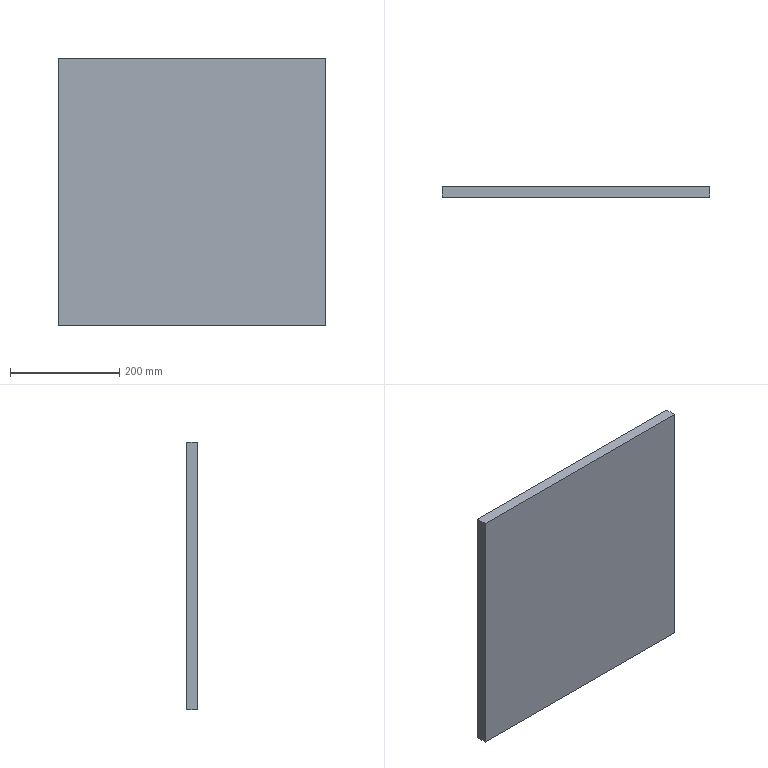Part | STEP file | 1 solid | 6 faces | box 490 x 20 x 490 mm | volume 4802000 mm3 | plane 6
STEP:
#1=CARTESIAN_POINT('',(0.,0.,0.));
#2=DIRECTION('',(0.,0.,1.));
#3=DIRECTION('',(1.,0.,0.));
#4=AXIS2_PLACEMENT_3D('',#1,#2,#3);
#5=CARTESIAN_POINT('',(245.,0.,245.));
#6=VERTEX_POINT('',#5);
#7=CARTESIAN_POINT('',(245.,0.,-245.));
#8=VERTEX_POINT('',#7);
#9=CARTESIAN_POINT('',(245.,0.,-245.));
#10=DIRECTION('',(0.,0.,-1.));
#11=VECTOR('',#10,1.);
#12=LINE('',#9,#11);
#13=CARTESIAN_POINT('',(245.,20.,-245.));
#14=DIRECTION('',(-1.,0.,0.));
#15=DIRECTION('',(0.,0.,1.));
#16=AXIS2_PLACEMENT_3D('',#13,#14,#15);
#17=PLANE('',#16);
#18=CARTESIAN_POINT('',(0.,-20.));
#19=DIRECTION('',(-1.,0.));
#20=VECTOR('',#19,1.);
#21=LINE('',#18,#20);
#22=(GEOMETRIC_REPRESENTATION_CONTEXT(2)PARAMETRIC_REPRESENTATION_CONTEXT()REPRESENTATION_CONTEXT('',''));
#23=DEFINITIONAL_REPRESENTATION('',(#21),#22);
#24=PCURVE('',#17,#23);
#25=CARTESIAN_POINT('',(0.,0.,0.));
#26=DIRECTION('',(0.,1.,0.));
#27=DIRECTION('',(0.,0.,1.));
#28=AXIS2_PLACEMENT_3D('',#25,#26,#27);
#29=PLANE('',#28);
#30=CARTESIAN_POINT('',(-245.,245.));
#31=DIRECTION('',(-1.,0.));
#32=VECTOR('',#31,1.);
#33=LINE('',#30,#32);
#34=(GEOMETRIC_REPRESENTATION_CONTEXT(2)PARAMETRIC_REPRESENTATION_CONTEXT()REPRESENTATION_CONTEXT('',''));
#35=DEFINITIONAL_REPRESENTATION('',(#33),#34);
#36=PCURVE('',#29,#35);
#37=SURFACE_CURVE('',#12,(#24,#36),.PCURVE_S1.);
#38=EDGE_CURVE('',#6,#8,#37,.T.);
#39=ORIENTED_EDGE('',*,*,#38,.T.);
#40=CARTESIAN_POINT('',(245.,20.,-245.));
#41=VERTEX_POINT('',#40);
#42=CARTESIAN_POINT('',(245.,20.,-245.));
#43=DIRECTION('',(0.,-1.,0.));
#44=VECTOR('',#43,1.);
#45=LINE('',#42,#44);
#46=CARTESIAN_POINT('',(0.,0.));
#47=DIRECTION('',(0.,-1.));
#48=VECTOR('',#47,1.);
#49=LINE('',#46,#48);
#50=(GEOMETRIC_REPRESENTATION_CONTEXT(2)PARAMETRIC_REPRESENTATION_CONTEXT()REPRESENTATION_CONTEXT('',''));
#51=DEFINITIONAL_REPRESENTATION('',(#49),#50);
#52=PCURVE('',#17,#51);
#53=CARTESIAN_POINT('',(-245.,20.,-245.));
#54=DIRECTION('',(0.,0.,1.));
#55=DIRECTION('',(1.,0.,0.));
#56=AXIS2_PLACEMENT_3D('',#53,#54,#55);
#57=PLANE('',#56);
#58=CARTESIAN_POINT('',(490.,0.));
#59=DIRECTION('',(0.,-1.));
#60=VECTOR('',#59,1.);
#61=LINE('',#58,#60);
#62=(GEOMETRIC_REPRESENTATION_CONTEXT(2)PARAMETRIC_REPRESENTATION_CONTEXT()REPRESENTATION_CONTEXT('',''));
#63=DEFINITIONAL_REPRESENTATION('',(#61),#62);
#64=PCURVE('',#57,#63);
#65=SURFACE_CURVE('',#45,(#52,#64),.PCURVE_S1.);
#66=EDGE_CURVE('',#41,#8,#65,.T.);
#67=ORIENTED_EDGE('',*,*,#66,.F.);
#68=CARTESIAN_POINT('',(245.,20.,245.));
#69=VERTEX_POINT('',#68);
#70=CARTESIAN_POINT('',(245.,20.,-245.));
#71=DIRECTION('',(0.,0.,-1.));
#72=VECTOR('',#71,1.);
#73=LINE('',#70,#72);
#74=CARTESIAN_POINT('',(0.,0.));
#75=DIRECTION('',(-1.,0.));
#76=VECTOR('',#75,1.);
#77=LINE('',#74,#76);
#78=(GEOMETRIC_REPRESENTATION_CONTEXT(2)PARAMETRIC_REPRESENTATION_CONTEXT()REPRESENTATION_CONTEXT('',''));
#79=DEFINITIONAL_REPRESENTATION('',(#77),#78);
#80=PCURVE('',#17,#79);
#81=CARTESIAN_POINT('',(0.,20.,0.));
#82=DIRECTION('',(0.,1.,0.));
#83=DIRECTION('',(0.,0.,1.));
#84=AXIS2_PLACEMENT_3D('',#81,#82,#83);
#85=PLANE('',#84);
#86=CARTESIAN_POINT('',(-245.,245.));
#87=DIRECTION('',(-1.,0.));
#88=VECTOR('',#87,1.);
#89=LINE('',#86,#88);
#90=(GEOMETRIC_REPRESENTATION_CONTEXT(2)PARAMETRIC_REPRESENTATION_CONTEXT()REPRESENTATION_CONTEXT('',''));
#91=DEFINITIONAL_REPRESENTATION('',(#89),#90);
#92=PCURVE('',#85,#91);
#93=SURFACE_CURVE('',#73,(#80,#92),.PCURVE_S1.);
#94=EDGE_CURVE('',#69,#41,#93,.T.);
#95=ORIENTED_EDGE('',*,*,#94,.F.);
#96=CARTESIAN_POINT('',(245.,20.,245.));
#97=DIRECTION('',(0.,-1.,0.));
#98=VECTOR('',#97,1.);
#99=LINE('',#96,#98);
#100=CARTESIAN_POINT('',(490.,0.));
#101=DIRECTION('',(0.,-1.));
#102=VECTOR('',#101,1.);
#103=LINE('',#100,#102);
#104=(GEOMETRIC_REPRESENTATION_CONTEXT(2)PARAMETRIC_REPRESENTATION_CONTEXT()REPRESENTATION_CONTEXT('',''));
#105=DEFINITIONAL_REPRESENTATION('',(#103),#104);
#106=PCURVE('',#17,#105);
#107=CARTESIAN_POINT('',(-245.,20.,245.));
#108=DIRECTION('',(0.,0.,-1.));
#109=DIRECTION('',(-1.,0.,0.));
#110=AXIS2_PLACEMENT_3D('',#107,#108,#109);
#111=PLANE('',#110);
#112=CARTESIAN_POINT('',(-490.,0.));
#113=DIRECTION('',(0.,-1.));
#114=VECTOR('',#113,1.);
#115=LINE('',#112,#114);
#116=(GEOMETRIC_REPRESENTATION_CONTEXT(2)PARAMETRIC_REPRESENTATION_CONTEXT()REPRESENTATION_CONTEXT('',''));
#117=DEFINITIONAL_REPRESENTATION('',(#115),#116);
#118=PCURVE('',#111,#117);
#119=SURFACE_CURVE('',#99,(#106,#118),.PCURVE_S1.);
#120=EDGE_CURVE('',#69,#6,#119,.T.);
#121=ORIENTED_EDGE('',*,*,#120,.T.);
#122=EDGE_LOOP('',(#39,#67,#95,#121));
#123=FACE_BOUND('',#122,.T.);
#124=ADVANCED_FACE('',(#123),#17,.F.);
#125=CARTESIAN_POINT('',(-245.,0.,-245.));
#126=VERTEX_POINT('',#125);
#127=CARTESIAN_POINT('',(-245.,0.,-245.));
#128=DIRECTION('',(-1.,0.,0.));
#129=VECTOR('',#128,1.);
#130=LINE('',#127,#129);
#131=CARTESIAN_POINT('',(0.,-20.));
#132=DIRECTION('',(-1.,0.));
#133=VECTOR('',#132,1.);
#134=LINE('',#131,#133);
#135=(GEOMETRIC_REPRESENTATION_CONTEXT(2)PARAMETRIC_REPRESENTATION_CONTEXT()REPRESENTATION_CONTEXT('',''));
#136=DEFINITIONAL_REPRESENTATION('',(#134),#135);
#137=PCURVE('',#57,#136);
#138=CARTESIAN_POINT('',(-245.,-245.));
#139=DIRECTION('',(0.,-1.));
#140=VECTOR('',#139,1.);
#141=LINE('',#138,#140);
#142=(GEOMETRIC_REPRESENTATION_CONTEXT(2)PARAMETRIC_REPRESENTATION_CONTEXT()REPRESENTATION_CONTEXT('',''));
#143=DEFINITIONAL_REPRESENTATION('',(#141),#142);
#144=PCURVE('',#29,#143);
#145=SURFACE_CURVE('',#130,(#137,#144),.PCURVE_S1.);
#146=EDGE_CURVE('',#8,#126,#145,.T.);
#147=ORIENTED_EDGE('',*,*,#146,.T.);
#148=CARTESIAN_POINT('',(-245.,20.,-245.));
#149=VERTEX_POINT('',#148);
#150=CARTESIAN_POINT('',(-245.,20.,-245.));
#151=DIRECTION('',(0.,-1.,0.));
#152=VECTOR('',#151,1.);
#153=LINE('',#150,#152);
#154=CARTESIAN_POINT('',(0.,0.));
#155=DIRECTION('',(0.,-1.));
#156=VECTOR('',#155,1.);
#157=LINE('',#154,#156);
#158=(GEOMETRIC_REPRESENTATION_CONTEXT(2)PARAMETRIC_REPRESENTATION_CONTEXT()REPRESENTATION_CONTEXT('',''));
#159=DEFINITIONAL_REPRESENTATION('',(#157),#158);
#160=PCURVE('',#57,#159);
#161=CARTESIAN_POINT('',(-245.,20.,-245.));
#162=DIRECTION('',(1.,0.,0.));
#163=DIRECTION('',(0.,0.,-1.));
#164=AXIS2_PLACEMENT_3D('',#161,#162,#163);
#165=PLANE('',#164);
#166=CARTESIAN_POINT('',(0.,0.));
#167=DIRECTION('',(0.,-1.));
#168=VECTOR('',#167,1.);
#169=LINE('',#166,#168);
#170=(GEOMETRIC_REPRESENTATION_CONTEXT(2)PARAMETRIC_REPRESENTATION_CONTEXT()REPRESENTATION_CONTEXT('',''));
#171=DEFINITIONAL_REPRESENTATION('',(#169),#170);
#172=PCURVE('',#165,#171);
#173=SURFACE_CURVE('',#153,(#160,#172),.PCURVE_S1.);
#174=EDGE_CURVE('',#149,#126,#173,.T.);
#175=ORIENTED_EDGE('',*,*,#174,.F.);
#176=CARTESIAN_POINT('',(-245.,20.,-245.));
#177=DIRECTION('',(-1.,0.,0.));
#178=VECTOR('',#177,1.);
#179=LINE('',#176,#178);
#180=CARTESIAN_POINT('',(0.,0.));
#181=DIRECTION('',(-1.,0.));
#182=VECTOR('',#181,1.);
#183=LINE('',#180,#182);
#184=(GEOMETRIC_REPRESENTATION_CONTEXT(2)PARAMETRIC_REPRESENTATION_CONTEXT()REPRESENTATION_CONTEXT('',''));
#185=DEFINITIONAL_REPRESENTATION('',(#183),#184);
#186=PCURVE('',#57,#185);
#187=CARTESIAN_POINT('',(-245.,-245.));
#188=DIRECTION('',(0.,-1.));
#189=VECTOR('',#188,1.);
#190=LINE('',#187,#189);
#191=(GEOMETRIC_REPRESENTATION_CONTEXT(2)PARAMETRIC_REPRESENTATION_CONTEXT()REPRESENTATION_CONTEXT('',''));
#192=DEFINITIONAL_REPRESENTATION('',(#190),#191);
#193=PCURVE('',#85,#192);
#194=SURFACE_CURVE('',#179,(#186,#193),.PCURVE_S1.);
#195=EDGE_CURVE('',#41,#149,#194,.T.);
#196=ORIENTED_EDGE('',*,*,#195,.F.);
#197=ORIENTED_EDGE('',*,*,#66,.T.);
#198=EDGE_LOOP('',(#147,#175,#196,#197));
#199=FACE_BOUND('',#198,.T.);
#200=ADVANCED_FACE('',(#199),#57,.F.);
#201=CARTESIAN_POINT('',(-245.,0.,245.));
#202=VERTEX_POINT('',#201);
#203=CARTESIAN_POINT('',(-245.,0.,-245.));
#204=DIRECTION('',(0.,0.,1.));
#205=VECTOR('',#204,1.);
#206=LINE('',#203,#205);
#207=CARTESIAN_POINT('',(0.,-20.));
#208=DIRECTION('',(-1.,0.));
#209=VECTOR('',#208,1.);
#210=LINE('',#207,#209);
#211=(GEOMETRIC_REPRESENTATION_CONTEXT(2)PARAMETRIC_REPRESENTATION_CONTEXT()REPRESENTATION_CONTEXT('',''));
#212=DEFINITIONAL_REPRESENTATION('',(#210),#211);
#213=PCURVE('',#165,#212);
#214=CARTESIAN_POINT('',(-245.,-245.));
#215=DIRECTION('',(1.,0.));
#216=VECTOR('',#215,1.);
#217=LINE('',#214,#216);
#218=(GEOMETRIC_REPRESENTATION_CONTEXT(2)PARAMETRIC_REPRESENTATION_CONTEXT()REPRESENTATION_CONTEXT('',''));
#219=DEFINITIONAL_REPRESENTATION('',(#217),#218);
#220=PCURVE('',#29,#219);
#221=SURFACE_CURVE('',#206,(#213,#220),.PCURVE_S1.);
#222=EDGE_CURVE('',#126,#202,#221,.T.);
#223=ORIENTED_EDGE('',*,*,#222,.T.);
#224=CARTESIAN_POINT('',(-245.,20.,245.));
#225=VERTEX_POINT('',#224);
#226=CARTESIAN_POINT('',(-245.,20.,245.));
#227=DIRECTION('',(0.,-1.,0.));
#228=VECTOR('',#227,1.);
#229=LINE('',#226,#228);
#230=CARTESIAN_POINT('',(-490.,0.));
#231=DIRECTION('',(0.,-1.));
#232=VECTOR('',#231,1.);
#233=LINE('',#230,#232);
#234=(GEOMETRIC_REPRESENTATION_CONTEXT(2)PARAMETRIC_REPRESENTATION_CONTEXT()REPRESENTATION_CONTEXT('',''));
#235=DEFINITIONAL_REPRESENTATION('',(#233),#234);
#236=PCURVE('',#165,#235);
#237=CARTESIAN_POINT('',(0.,0.));
#238=DIRECTION('',(0.,-1.));
#239=VECTOR('',#238,1.);
#240=LINE('',#237,#239);
#241=(GEOMETRIC_REPRESENTATION_CONTEXT(2)PARAMETRIC_REPRESENTATION_CONTEXT()REPRESENTATION_CONTEXT('',''));
#242=DEFINITIONAL_REPRESENTATION('',(#240),#241);
#243=PCURVE('',#111,#242);
#244=SURFACE_CURVE('',#229,(#236,#243),.PCURVE_S1.);
#245=EDGE_CURVE('',#225,#202,#244,.T.);
#246=ORIENTED_EDGE('',*,*,#245,.F.);
#247=CARTESIAN_POINT('',(-245.,20.,-245.));
#248=DIRECTION('',(0.,0.,1.));
#249=VECTOR('',#248,1.);
#250=LINE('',#247,#249);
#251=CARTESIAN_POINT('',(0.,0.));
#252=DIRECTION('',(-1.,0.));
#253=VECTOR('',#252,1.);
#254=LINE('',#251,#253);
#255=(GEOMETRIC_REPRESENTATION_CONTEXT(2)PARAMETRIC_REPRESENTATION_CONTEXT()REPRESENTATION_CONTEXT('',''));
#256=DEFINITIONAL_REPRESENTATION('',(#254),#255);
#257=PCURVE('',#165,#256);
#258=CARTESIAN_POINT('',(-245.,-245.));
#259=DIRECTION('',(1.,0.));
#260=VECTOR('',#259,1.);
#261=LINE('',#258,#260);
#262=(GEOMETRIC_REPRESENTATION_CONTEXT(2)PARAMETRIC_REPRESENTATION_CONTEXT()REPRESENTATION_CONTEXT('',''));
#263=DEFINITIONAL_REPRESENTATION('',(#261),#262);
#264=PCURVE('',#85,#263);
#265=SURFACE_CURVE('',#250,(#257,#264),.PCURVE_S1.);
#266=EDGE_CURVE('',#149,#225,#265,.T.);
#267=ORIENTED_EDGE('',*,*,#266,.F.);
#268=ORIENTED_EDGE('',*,*,#174,.T.);
#269=EDGE_LOOP('',(#223,#246,#267,#268));
#270=FACE_BOUND('',#269,.T.);
#271=ADVANCED_FACE('',(#270),#165,.F.);
#272=CARTESIAN_POINT('',(-245.,0.,245.));
#273=DIRECTION('',(1.,0.,0.));
#274=VECTOR('',#273,1.);
#275=LINE('',#272,#274);
#276=CARTESIAN_POINT('',(0.,-20.));
#277=DIRECTION('',(-1.,0.));
#278=VECTOR('',#277,1.);
#279=LINE('',#276,#278);
#280=(GEOMETRIC_REPRESENTATION_CONTEXT(2)PARAMETRIC_REPRESENTATION_CONTEXT()REPRESENTATION_CONTEXT('',''));
#281=DEFINITIONAL_REPRESENTATION('',(#279),#280);
#282=PCURVE('',#111,#281);
#283=CARTESIAN_POINT('',(245.,-245.));
#284=DIRECTION('',(0.,1.));
#285=VECTOR('',#284,1.);
#286=LINE('',#283,#285);
#287=(GEOMETRIC_REPRESENTATION_CONTEXT(2)PARAMETRIC_REPRESENTATION_CONTEXT()REPRESENTATION_CONTEXT('',''));
#288=DEFINITIONAL_REPRESENTATION('',(#286),#287);
#289=PCURVE('',#29,#288);
#290=SURFACE_CURVE('',#275,(#282,#289),.PCURVE_S1.);
#291=EDGE_CURVE('',#202,#6,#290,.T.);
#292=ORIENTED_EDGE('',*,*,#291,.T.);
#293=ORIENTED_EDGE('',*,*,#120,.F.);
#294=CARTESIAN_POINT('',(-245.,20.,245.));
#295=DIRECTION('',(1.,0.,0.));
#296=VECTOR('',#295,1.);
#297=LINE('',#294,#296);
#298=CARTESIAN_POINT('',(0.,0.));
#299=DIRECTION('',(-1.,0.));
#300=VECTOR('',#299,1.);
#301=LINE('',#298,#300);
#302=(GEOMETRIC_REPRESENTATION_CONTEXT(2)PARAMETRIC_REPRESENTATION_CONTEXT()REPRESENTATION_CONTEXT('',''));
#303=DEFINITIONAL_REPRESENTATION('',(#301),#302);
#304=PCURVE('',#111,#303);
#305=CARTESIAN_POINT('',(245.,-245.));
#306=DIRECTION('',(0.,1.));
#307=VECTOR('',#306,1.);
#308=LINE('',#305,#307);
#309=(GEOMETRIC_REPRESENTATION_CONTEXT(2)PARAMETRIC_REPRESENTATION_CONTEXT()REPRESENTATION_CONTEXT('',''));
#310=DEFINITIONAL_REPRESENTATION('',(#308),#309);
#311=PCURVE('',#85,#310);
#312=SURFACE_CURVE('',#297,(#304,#311),.PCURVE_S1.);
#313=EDGE_CURVE('',#225,#69,#312,.T.);
#314=ORIENTED_EDGE('',*,*,#313,.F.);
#315=ORIENTED_EDGE('',*,*,#245,.T.);
#316=EDGE_LOOP('',(#292,#293,#314,#315));
#317=FACE_BOUND('',#316,.T.);
#318=ADVANCED_FACE('',(#317),#111,.F.);
#319=ORIENTED_EDGE('',*,*,#94,.T.);
#320=ORIENTED_EDGE('',*,*,#195,.T.);
#321=ORIENTED_EDGE('',*,*,#266,.T.);
#322=ORIENTED_EDGE('',*,*,#313,.T.);
#323=EDGE_LOOP('',(#319,#320,#321,#322));
#324=FACE_BOUND('',#323,.T.);
#325=ADVANCED_FACE('',(#324),#85,.T.);
#326=ORIENTED_EDGE('',*,*,#38,.F.);
#327=ORIENTED_EDGE('',*,*,#291,.F.);
#328=ORIENTED_EDGE('',*,*,#222,.F.);
#329=ORIENTED_EDGE('',*,*,#146,.F.);
#330=EDGE_LOOP('',(#326,#327,#328,#329));
#331=FACE_BOUND('',#330,.T.);
#332=ADVANCED_FACE('',(#331),#29,.F.);
#333=CLOSED_SHELL('',(#124,#200,#271,#318,#325,#332));
#334=MANIFOLD_SOLID_BREP('',#333);
#335=(LENGTH_UNIT()NAMED_UNIT(*)SI_UNIT(.MILLI.,.METRE.));
#336=UNCERTAINTY_MEASURE_WITH_UNIT(LENGTH_MEASURE(0.0000001),#335,'','');
#337=(NAMED_UNIT(*)PLANE_ANGLE_UNIT()SI_UNIT($,.RADIAN.));
#338=(NAMED_UNIT(*)SI_UNIT($,.STERADIAN.)SOLID_ANGLE_UNIT());
#339=(GEOMETRIC_REPRESENTATION_CONTEXT(3)GLOBAL_UNCERTAINTY_ASSIGNED_CONTEXT((#336))GLOBAL_UNIT_ASSIGNED_CONTEXT((#335,#337,#338))REPRESENTATION_CONTEXT('',''));
#340=ADVANCED_BREP_SHAPE_REPRESENTATION('',(#4,#334),#339);